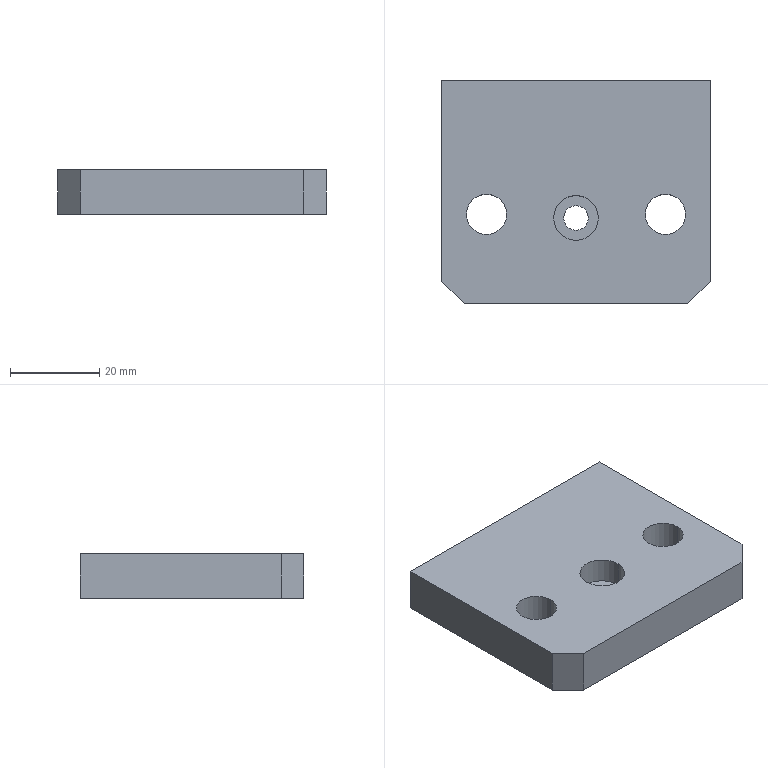Part | SolidWorks | features BaseBody 1 | 1 solid | 29 faces | box 60 x 50 x 10 mm | volume 27328 mm3 | cylinder 14 | plane 9 | cone 6 | commonest cylinder face diameters 4.2 x6 9 x4 5.5 x2 10 x2
STEP:
#1=CARTESIAN_POINT('',(-5.,-5.8,4.3));
#2=VERTEX_POINT('',#1);
#3=CARTESIAN_POINT('',(5.,-5.8,4.3));
#4=VERTEX_POINT('',#3);
#5=CARTESIAN_POINT('',(0.,-5.8,4.3));
#6=DIRECTION('',(0.,0.,1.));
#7=DIRECTION('',(1.,0.,0.));
#8=AXIS2_PLACEMENT_3D('',#5,#6,#7);
#9=CIRCLE('',#8,5.);
#10=EDGE_CURVE('',#2,#4,#9,.T.);
#11=ORIENTED_EDGE('',*,*,#10,.F.);
#12=CARTESIAN_POINT('',(-5.,-5.8,10.));
#13=VERTEX_POINT('',#12);
#14=CARTESIAN_POINT('',(-5.,-5.8,10.));
#15=DIRECTION('',(0.,0.,1.));
#16=VECTOR('',#15,1000.);
#17=LINE('',#14,#16);
#18=EDGE_CURVE('',#2,#13,#17,.T.);
#19=ORIENTED_EDGE('',*,*,#18,.T.);
#20=CARTESIAN_POINT('',(5.,-5.8,10.));
#21=VERTEX_POINT('',#20);
#22=CARTESIAN_POINT('',(0.,-5.8,10.));
#23=DIRECTION('',(0.,0.,1.));
#24=DIRECTION('',(1.,0.,0.));
#25=AXIS2_PLACEMENT_3D('',#22,#23,#24);
#26=CIRCLE('',#25,5.);
#27=EDGE_CURVE('',#13,#21,#26,.T.);
#28=ORIENTED_EDGE('',*,*,#27,.T.);
#29=CARTESIAN_POINT('',(5.,-5.8,10.));
#30=DIRECTION('',(0.,0.,1.));
#31=VECTOR('',#30,1000.);
#32=LINE('',#29,#31);
#33=EDGE_CURVE('',#4,#21,#32,.T.);
#34=ORIENTED_EDGE('',*,*,#33,.F.);
#35=EDGE_LOOP('',(#11,#19,#28,#34));
#36=FACE_OUTER_BOUND('',#35,.T.);
#37=CARTESIAN_POINT('',(0.,-5.8,10.));
#38=DIRECTION('',(0.,0.,1.));
#39=DIRECTION('',(1.,0.,0.));
#40=AXIS2_PLACEMENT_3D('',#37,#38,#39);
#41=CYLINDRICAL_SURFACE('',#40,5.);
#42=ADVANCED_FACE('',(#36),#41,.F.);
#43=CARTESIAN_POINT('',(-2.75,-5.8,0.));
#44=VERTEX_POINT('',#43);
#45=CARTESIAN_POINT('',(2.75,-5.8,0.));
#46=VERTEX_POINT('',#45);
#47=CARTESIAN_POINT('',(0.,-5.8,0.));
#48=DIRECTION('',(0.,0.,1.));
#49=DIRECTION('',(1.,0.,0.));
#50=AXIS2_PLACEMENT_3D('',#47,#48,#49);
#51=CIRCLE('',#50,2.75);
#52=EDGE_CURVE('',#44,#46,#51,.T.);
#53=ORIENTED_EDGE('',*,*,#52,.F.);
#54=CARTESIAN_POINT('',(-2.75,-5.8,4.3));
#55=VERTEX_POINT('',#54);
#56=CARTESIAN_POINT('',(-2.75,-5.8,10.));
#57=DIRECTION('',(0.,0.,1.));
#58=VECTOR('',#57,1000.);
#59=LINE('',#56,#58);
#60=EDGE_CURVE('',#44,#55,#59,.T.);
#61=ORIENTED_EDGE('',*,*,#60,.T.);
#62=CARTESIAN_POINT('',(2.75,-5.8,4.3));
#63=VERTEX_POINT('',#62);
#64=CARTESIAN_POINT('',(0.,-5.8,4.3));
#65=DIRECTION('',(0.,0.,1.));
#66=DIRECTION('',(1.,0.,0.));
#67=AXIS2_PLACEMENT_3D('',#64,#65,#66);
#68=CIRCLE('',#67,2.75);
#69=EDGE_CURVE('',#55,#63,#68,.T.);
#70=ORIENTED_EDGE('',*,*,#69,.T.);
#71=CARTESIAN_POINT('',(2.75,-5.8,10.));
#72=DIRECTION('',(0.,0.,1.));
#73=VECTOR('',#72,1000.);
#74=LINE('',#71,#73);
#75=EDGE_CURVE('',#46,#63,#74,.T.);
#76=ORIENTED_EDGE('',*,*,#75,.F.);
#77=EDGE_LOOP('',(#53,#61,#70,#76));
#78=FACE_OUTER_BOUND('',#77,.T.);
#79=CARTESIAN_POINT('',(0.,-5.8,10.));
#80=DIRECTION('',(0.,0.,1.));
#81=DIRECTION('',(1.,0.,0.));
#82=AXIS2_PLACEMENT_3D('',#79,#80,#81);
#83=CYLINDRICAL_SURFACE('',#82,2.75);
#84=ADVANCED_FACE('',(#78),#83,.F.);
#85=CARTESIAN_POINT('',(-20.,11.,2.9));
#86=VERTEX_POINT('',#85);
#87=CARTESIAN_POINT('',(-20.,11.,7.1));
#88=VERTEX_POINT('',#87);
#89=CARTESIAN_POINT('',(-20.,11.,5.));
#90=DIRECTION('',(0.,1.,0.));
#91=DIRECTION('',(0.,0.,1.));
#92=AXIS2_PLACEMENT_3D('',#89,#90,#91);
#93=CIRCLE('',#92,2.1);
#94=EDGE_CURVE('',#86,#88,#93,.T.);
#95=ORIENTED_EDGE('',*,*,#94,.F.);
#96=CARTESIAN_POINT('',(-20.,25.,2.9));
#97=VERTEX_POINT('',#96);
#98=CARTESIAN_POINT('',(-20.,25.,2.9));
#99=DIRECTION('',(0.,1.,0.));
#100=VECTOR('',#99,1000.);
#101=LINE('',#98,#100);
#102=EDGE_CURVE('',#86,#97,#101,.T.);
#103=ORIENTED_EDGE('',*,*,#102,.T.);
#104=CARTESIAN_POINT('',(-20.,25.,7.1));
#105=VERTEX_POINT('',#104);
#106=CARTESIAN_POINT('',(-20.,25.,5.));
#107=DIRECTION('',(0.,1.,0.));
#108=DIRECTION('',(0.,0.,1.));
#109=AXIS2_PLACEMENT_3D('',#106,#107,#108);
#110=CIRCLE('',#109,2.1);
#111=EDGE_CURVE('',#97,#105,#110,.T.);
#112=ORIENTED_EDGE('',*,*,#111,.T.);
#113=CARTESIAN_POINT('',(-20.,25.,7.1));
#114=DIRECTION('',(0.,1.,0.));
#115=VECTOR('',#114,1000.);
#116=LINE('',#113,#115);
#117=EDGE_CURVE('',#88,#105,#116,.T.);
#118=ORIENTED_EDGE('',*,*,#117,.F.);
#119=EDGE_LOOP('',(#95,#103,#112,#118));
#120=FACE_OUTER_BOUND('',#119,.T.);
#121=CARTESIAN_POINT('',(-20.,25.,5.));
#122=DIRECTION('',(0.,1.,0.));
#123=DIRECTION('',(0.,0.,1.));
#124=AXIS2_PLACEMENT_3D('',#121,#122,#123);
#125=CYLINDRICAL_SURFACE('',#124,2.1);
#126=ADVANCED_FACE('',(#120),#125,.F.);
#127=CARTESIAN_POINT('',(-20.,9.738,5.));
#128=VERTEX_POINT('',#127);
#129=CARTESIAN_POINT('',(-20.,11.,7.1));
#130=DIRECTION('',(0.,0.515,0.8572));
#131=VECTOR('',#130,1000.);
#132=LINE('',#129,#131);
#133=EDGE_CURVE('',#128,#88,#132,.T.);
#134=ORIENTED_EDGE('',*,*,#133,.F.);
#135=CARTESIAN_POINT('',(-20.,11.,2.9));
#136=DIRECTION('',(0.,0.515,-0.8572));
#137=VECTOR('',#136,1000.);
#138=LINE('',#135,#137);
#139=EDGE_CURVE('',#128,#86,#138,.T.);
#140=ORIENTED_EDGE('',*,*,#139,.T.);
#141=ORIENTED_EDGE('',*,*,#94,.T.);
#142=EDGE_LOOP('',(#134,#140,#141));
#143=FACE_OUTER_BOUND('',#142,.T.);
#144=CARTESIAN_POINT('',(-20.,11.,5.));
#145=DIRECTION('',(0.,1.,0.));
#146=DIRECTION('',(0.,0.,1.));
#147=AXIS2_PLACEMENT_3D('',#144,#145,#146);
#148=CONICAL_SURFACE('',#147,2.1,1.03);
#149=ADVANCED_FACE('',(#143),#148,.F.);
#150=CARTESIAN_POINT('',(0.,11.,2.9));
#151=VERTEX_POINT('',#150);
#152=CARTESIAN_POINT('',(0.,11.,7.1));
#153=VERTEX_POINT('',#152);
#154=CARTESIAN_POINT('',(0.,11.,5.));
#155=DIRECTION('',(0.,1.,0.));
#156=DIRECTION('',(0.,0.,1.));
#157=AXIS2_PLACEMENT_3D('',#154,#155,#156);
#158=CIRCLE('',#157,2.1);
#159=EDGE_CURVE('',#151,#153,#158,.T.);
#160=ORIENTED_EDGE('',*,*,#159,.F.);
#161=CARTESIAN_POINT('',(0.,25.,2.9));
#162=VERTEX_POINT('',#161);
#163=CARTESIAN_POINT('',(0.,25.,2.9));
#164=DIRECTION('',(0.,1.,0.));
#165=VECTOR('',#164,1000.);
#166=LINE('',#163,#165);
#167=EDGE_CURVE('',#151,#162,#166,.T.);
#168=ORIENTED_EDGE('',*,*,#167,.T.);
#169=CARTESIAN_POINT('',(0.,25.,7.1));
#170=VERTEX_POINT('',#169);
#171=CARTESIAN_POINT('',(0.,25.,5.));
#172=DIRECTION('',(0.,1.,0.));
#173=DIRECTION('',(0.,0.,1.));
#174=AXIS2_PLACEMENT_3D('',#171,#172,#173);
#175=CIRCLE('',#174,2.1);
#176=EDGE_CURVE('',#162,#170,#175,.T.);
#177=ORIENTED_EDGE('',*,*,#176,.T.);
#178=CARTESIAN_POINT('',(0.,25.,7.1));
#179=DIRECTION('',(0.,1.,0.));
#180=VECTOR('',#179,1000.);
#181=LINE('',#178,#180);
#182=EDGE_CURVE('',#153,#170,#181,.T.);
#183=ORIENTED_EDGE('',*,*,#182,.F.);
#184=EDGE_LOOP('',(#160,#168,#177,#183));
#185=FACE_OUTER_BOUND('',#184,.T.);
#186=CARTESIAN_POINT('',(0.,25.,5.));
#187=DIRECTION('',(0.,1.,0.));
#188=DIRECTION('',(0.,0.,1.));
#189=AXIS2_PLACEMENT_3D('',#186,#187,#188);
#190=CYLINDRICAL_SURFACE('',#189,2.1);
#191=ADVANCED_FACE('',(#185),#190,.F.);
#192=CARTESIAN_POINT('',(0.,9.738,5.));
#193=VERTEX_POINT('',#192);
#194=CARTESIAN_POINT('',(0.,11.,7.1));
#195=DIRECTION('',(0.,0.515,0.8572));
#196=VECTOR('',#195,1000.);
#197=LINE('',#194,#196);
#198=EDGE_CURVE('',#193,#153,#197,.T.);
#199=ORIENTED_EDGE('',*,*,#198,.F.);
#200=CARTESIAN_POINT('',(0.,11.,2.9));
#201=DIRECTION('',(0.,0.515,-0.8572));
#202=VECTOR('',#201,1000.);
#203=LINE('',#200,#202);
#204=EDGE_CURVE('',#193,#151,#203,.T.);
#205=ORIENTED_EDGE('',*,*,#204,.T.);
#206=ORIENTED_EDGE('',*,*,#159,.T.);
#207=EDGE_LOOP('',(#199,#205,#206));
#208=FACE_OUTER_BOUND('',#207,.T.);
#209=CARTESIAN_POINT('',(0.,11.,5.));
#210=DIRECTION('',(0.,1.,0.));
#211=DIRECTION('',(0.,0.,1.));
#212=AXIS2_PLACEMENT_3D('',#209,#210,#211);
#213=CONICAL_SURFACE('',#212,2.1,1.03);
#214=ADVANCED_FACE('',(#208),#213,.F.);
#215=CARTESIAN_POINT('',(20.,11.,2.9));
#216=VERTEX_POINT('',#215);
#217=CARTESIAN_POINT('',(20.,11.,7.1));
#218=VERTEX_POINT('',#217);
#219=CARTESIAN_POINT('',(20.,11.,5.));
#220=DIRECTION('',(0.,1.,0.));
#221=DIRECTION('',(0.,0.,1.));
#222=AXIS2_PLACEMENT_3D('',#219,#220,#221);
#223=CIRCLE('',#222,2.1);
#224=EDGE_CURVE('',#216,#218,#223,.T.);
#225=ORIENTED_EDGE('',*,*,#224,.F.);
#226=CARTESIAN_POINT('',(20.,25.,2.9));
#227=VERTEX_POINT('',#226);
#228=CARTESIAN_POINT('',(20.,25.,2.9));
#229=DIRECTION('',(0.,1.,0.));
#230=VECTOR('',#229,1000.);
#231=LINE('',#228,#230);
#232=EDGE_CURVE('',#216,#227,#231,.T.);
#233=ORIENTED_EDGE('',*,*,#232,.T.);
#234=CARTESIAN_POINT('',(20.,25.,7.1));
#235=VERTEX_POINT('',#234);
#236=CARTESIAN_POINT('',(20.,25.,5.));
#237=DIRECTION('',(0.,1.,0.));
#238=DIRECTION('',(0.,0.,1.));
#239=AXIS2_PLACEMENT_3D('',#236,#237,#238);
#240=CIRCLE('',#239,2.1);
#241=EDGE_CURVE('',#227,#235,#240,.T.);
#242=ORIENTED_EDGE('',*,*,#241,.T.);
#243=CARTESIAN_POINT('',(20.,25.,7.1));
#244=DIRECTION('',(0.,1.,0.));
#245=VECTOR('',#244,1000.);
#246=LINE('',#243,#245);
#247=EDGE_CURVE('',#218,#235,#246,.T.);
#248=ORIENTED_EDGE('',*,*,#247,.F.);
#249=EDGE_LOOP('',(#225,#233,#242,#248));
#250=FACE_OUTER_BOUND('',#249,.T.);
#251=CARTESIAN_POINT('',(20.,25.,5.));
#252=DIRECTION('',(0.,1.,0.));
#253=DIRECTION('',(0.,0.,1.));
#254=AXIS2_PLACEMENT_3D('',#251,#252,#253);
#255=CYLINDRICAL_SURFACE('',#254,2.1);
#256=ADVANCED_FACE('',(#250),#255,.F.);
#257=CARTESIAN_POINT('',(20.,9.738,5.));
#258=VERTEX_POINT('',#257);
#259=CARTESIAN_POINT('',(20.,11.,7.1));
#260=DIRECTION('',(0.,0.515,0.8572));
#261=VECTOR('',#260,1000.);
#262=LINE('',#259,#261);
#263=EDGE_CURVE('',#258,#218,#262,.T.);
#264=ORIENTED_EDGE('',*,*,#263,.F.);
#265=CARTESIAN_POINT('',(20.,11.,2.9));
#266=DIRECTION('',(0.,0.515,-0.8572));
#267=VECTOR('',#266,1000.);
#268=LINE('',#265,#267);
#269=EDGE_CURVE('',#258,#216,#268,.T.);
#270=ORIENTED_EDGE('',*,*,#269,.T.);
#271=ORIENTED_EDGE('',*,*,#224,.T.);
#272=EDGE_LOOP('',(#264,#270,#271));
#273=FACE_OUTER_BOUND('',#272,.T.);
#274=CARTESIAN_POINT('',(20.,11.,5.));
#275=DIRECTION('',(0.,1.,0.));
#276=DIRECTION('',(0.,0.,1.));
#277=AXIS2_PLACEMENT_3D('',#274,#275,#276);
#278=CONICAL_SURFACE('',#277,2.1,1.03);
#279=ADVANCED_FACE('',(#273),#278,.F.);
#280=CARTESIAN_POINT('',(-24.5,-5.,0.));
#281=VERTEX_POINT('',#280);
#282=CARTESIAN_POINT('',(-15.5,-5.,0.));
#283=VERTEX_POINT('',#282);
#284=CARTESIAN_POINT('',(-20.,-5.,0.));
#285=DIRECTION('',(0.,0.,1.));
#286=DIRECTION('',(1.,0.,0.));
#287=AXIS2_PLACEMENT_3D('',#284,#285,#286);
#288=CIRCLE('',#287,4.5);
#289=EDGE_CURVE('',#281,#283,#288,.T.);
#290=ORIENTED_EDGE('',*,*,#289,.F.);
#291=CARTESIAN_POINT('',(-24.5,-5.,10.));
#292=VERTEX_POINT('',#291);
#293=CARTESIAN_POINT('',(-24.5,-5.,10.));
#294=DIRECTION('',(0.,0.,1.));
#295=VECTOR('',#294,1000.);
#296=LINE('',#293,#295);
#297=EDGE_CURVE('',#281,#292,#296,.T.);
#298=ORIENTED_EDGE('',*,*,#297,.T.);
#299=CARTESIAN_POINT('',(-15.5,-5.,10.));
#300=VERTEX_POINT('',#299);
#301=CARTESIAN_POINT('',(-20.,-5.,10.));
#302=DIRECTION('',(0.,0.,1.));
#303=DIRECTION('',(1.,0.,0.));
#304=AXIS2_PLACEMENT_3D('',#301,#302,#303);
#305=CIRCLE('',#304,4.5);
#306=EDGE_CURVE('',#292,#300,#305,.T.);
#307=ORIENTED_EDGE('',*,*,#306,.T.);
#308=CARTESIAN_POINT('',(-15.5,-5.,10.));
#309=DIRECTION('',(0.,0.,1.));
#310=VECTOR('',#309,1000.);
#311=LINE('',#308,#310);
#312=EDGE_CURVE('',#283,#300,#311,.T.);
#313=ORIENTED_EDGE('',*,*,#312,.F.);
#314=EDGE_LOOP('',(#290,#298,#307,#313));
#315=FACE_OUTER_BOUND('',#314,.T.);
#316=CARTESIAN_POINT('',(-20.,-5.,10.));
#317=DIRECTION('',(0.,0.,1.));
#318=DIRECTION('',(1.,0.,0.));
#319=AXIS2_PLACEMENT_3D('',#316,#317,#318);
#320=CYLINDRICAL_SURFACE('',#319,4.5);
#321=ADVANCED_FACE('',(#315),#320,.F.);
#322=CARTESIAN_POINT('',(15.5,-5.,0.));
#323=VERTEX_POINT('',#322);
#324=CARTESIAN_POINT('',(24.5,-5.,0.));
#325=VERTEX_POINT('',#324);
#326=CARTESIAN_POINT('',(20.,-5.,0.));
#327=DIRECTION('',(0.,0.,1.));
#328=DIRECTION('',(1.,0.,0.));
#329=AXIS2_PLACEMENT_3D('',#326,#327,#328);
#330=CIRCLE('',#329,4.5);
#331=EDGE_CURVE('',#323,#325,#330,.T.);
#332=ORIENTED_EDGE('',*,*,#331,.F.);
#333=CARTESIAN_POINT('',(15.5,-5.,10.));
#334=VERTEX_POINT('',#333);
#335=CARTESIAN_POINT('',(15.5,-5.,10.));
#336=DIRECTION('',(0.,0.,1.));
#337=VECTOR('',#336,1000.);
#338=LINE('',#335,#337);
#339=EDGE_CURVE('',#323,#334,#338,.T.);
#340=ORIENTED_EDGE('',*,*,#339,.T.);
#341=CARTESIAN_POINT('',(24.5,-5.,10.));
#342=VERTEX_POINT('',#341);
#343=CARTESIAN_POINT('',(20.,-5.,10.));
#344=DIRECTION('',(0.,0.,1.));
#345=DIRECTION('',(1.,0.,0.));
#346=AXIS2_PLACEMENT_3D('',#343,#344,#345);
#347=CIRCLE('',#346,4.5);
#348=EDGE_CURVE('',#334,#342,#347,.T.);
#349=ORIENTED_EDGE('',*,*,#348,.T.);
#350=CARTESIAN_POINT('',(24.5,-5.,10.));
#351=DIRECTION('',(0.,0.,1.));
#352=VECTOR('',#351,1000.);
#353=LINE('',#350,#352);
#354=EDGE_CURVE('',#325,#342,#353,.T.);
#355=ORIENTED_EDGE('',*,*,#354,.F.);
#356=EDGE_LOOP('',(#332,#340,#349,#355));
#357=FACE_OUTER_BOUND('',#356,.T.);
#358=CARTESIAN_POINT('',(20.,-5.,10.));
#359=DIRECTION('',(0.,0.,1.));
#360=DIRECTION('',(1.,0.,0.));
#361=AXIS2_PLACEMENT_3D('',#358,#359,#360);
#362=CYLINDRICAL_SURFACE('',#361,4.5);
#363=ADVANCED_FACE('',(#357),#362,.F.);
#364=CARTESIAN_POINT('',(-30.,25.,0.));
#365=VERTEX_POINT('',#364);
#366=CARTESIAN_POINT('',(-30.,-20.,0.));
#367=VERTEX_POINT('',#366);
#368=CARTESIAN_POINT('',(-30.,25.,0.));
#369=DIRECTION('',(0.,-1.,0.));
#370=VECTOR('',#369,1000.);
#371=LINE('',#368,#370);
#372=EDGE_CURVE('',#365,#367,#371,.T.);
#373=ORIENTED_EDGE('',*,*,#372,.T.);
#374=CARTESIAN_POINT('',(-30.,-20.,10.));
#375=VERTEX_POINT('',#374);
#376=CARTESIAN_POINT('',(-30.,-20.,10.));
#377=DIRECTION('',(0.,0.,1.));
#378=VECTOR('',#377,1000.);
#379=LINE('',#376,#378);
#380=EDGE_CURVE('',#367,#375,#379,.T.);
#381=ORIENTED_EDGE('',*,*,#380,.T.);
#382=CARTESIAN_POINT('',(-30.,25.,10.));
#383=VERTEX_POINT('',#382);
#384=CARTESIAN_POINT('',(-30.,25.,10.));
#385=DIRECTION('',(0.,-1.,0.));
#386=VECTOR('',#385,1000.);
#387=LINE('',#384,#386);
#388=EDGE_CURVE('',#383,#375,#387,.T.);
#389=ORIENTED_EDGE('',*,*,#388,.F.);
#390=CARTESIAN_POINT('',(-30.,25.,10.));
#391=DIRECTION('',(0.,0.,-1.));
#392=VECTOR('',#391,1000.);
#393=LINE('',#390,#392);
#394=EDGE_CURVE('',#383,#365,#393,.T.);
#395=ORIENTED_EDGE('',*,*,#394,.T.);
#396=EDGE_LOOP('',(#373,#381,#389,#395));
#397=FACE_OUTER_BOUND('',#396,.T.);
#398=CARTESIAN_POINT('',(-30.,25.,10.));
#399=DIRECTION('',(1.,0.,0.));
#400=DIRECTION('',(0.,1.,0.));
#401=AXIS2_PLACEMENT_3D('',#398,#399,#400);
#402=PLANE('',#401);
#403=ADVANCED_FACE('',(#397),#402,.F.);
#404=CARTESIAN_POINT('',(-25.,-25.,10.));
#405=VERTEX_POINT('',#404);
#406=CARTESIAN_POINT('',(25.,-25.,10.));
#407=VERTEX_POINT('',#406);
#408=CARTESIAN_POINT('',(30.,-25.,10.));
#409=DIRECTION('',(1.,0.,0.));
#410=VECTOR('',#409,1000.);
#411=LINE('',#408,#410);
#412=EDGE_CURVE('',#405,#407,#411,.T.);
#413=ORIENTED_EDGE('',*,*,#412,.F.);
#414=CARTESIAN_POINT('',(-25.,-25.,0.));
#415=VERTEX_POINT('',#414);
#416=CARTESIAN_POINT('',(-25.,-25.,10.));
#417=DIRECTION('',(0.,0.,-1.));
#418=VECTOR('',#417,1000.);
#419=LINE('',#416,#418);
#420=EDGE_CURVE('',#405,#415,#419,.T.);
#421=ORIENTED_EDGE('',*,*,#420,.T.);
#422=CARTESIAN_POINT('',(25.,-25.,0.));
#423=VERTEX_POINT('',#422);
#424=CARTESIAN_POINT('',(30.,-25.,0.));
#425=DIRECTION('',(1.,0.,0.));
#426=VECTOR('',#425,1000.);
#427=LINE('',#424,#426);
#428=EDGE_CURVE('',#415,#423,#427,.T.);
#429=ORIENTED_EDGE('',*,*,#428,.T.);
#430=CARTESIAN_POINT('',(25.,-25.,10.));
#431=DIRECTION('',(0.,0.,1.));
#432=VECTOR('',#431,1000.);
#433=LINE('',#430,#432);
#434=EDGE_CURVE('',#423,#407,#433,.T.);
#435=ORIENTED_EDGE('',*,*,#434,.T.);
#436=EDGE_LOOP('',(#413,#421,#429,#435));
#437=FACE_OUTER_BOUND('',#436,.T.);
#438=CARTESIAN_POINT('',(30.,-25.,10.));
#439=DIRECTION('',(0.,1.,0.));
#440=DIRECTION('',(-1.,0.,0.));
#441=AXIS2_PLACEMENT_3D('',#438,#439,#440);
#442=PLANE('',#441);
#443=ADVANCED_FACE('',(#437),#442,.F.);
#444=CARTESIAN_POINT('',(30.,-20.,10.));
#445=VERTEX_POINT('',#444);
#446=CARTESIAN_POINT('',(30.,25.,10.));
#447=VERTEX_POINT('',#446);
#448=CARTESIAN_POINT('',(30.,25.,10.));
#449=DIRECTION('',(0.,1.,0.));
#450=VECTOR('',#449,1000.);
#451=LINE('',#448,#450);
#452=EDGE_CURVE('',#445,#447,#451,.T.);
#453=ORIENTED_EDGE('',*,*,#452,.F.);
#454=CARTESIAN_POINT('',(30.,-20.,0.));
#455=VERTEX_POINT('',#454);
#456=CARTESIAN_POINT('',(30.,-20.,10.));
#457=DIRECTION('',(0.,0.,-1.));
#458=VECTOR('',#457,1000.);
#459=LINE('',#456,#458);
#460=EDGE_CURVE('',#445,#455,#459,.T.);
#461=ORIENTED_EDGE('',*,*,#460,.T.);
#462=CARTESIAN_POINT('',(30.,25.,0.));
#463=VERTEX_POINT('',#462);
#464=CARTESIAN_POINT('',(30.,25.,0.));
#465=DIRECTION('',(0.,1.,0.));
#466=VECTOR('',#465,1000.);
#467=LINE('',#464,#466);
#468=EDGE_CURVE('',#455,#463,#467,.T.);
#469=ORIENTED_EDGE('',*,*,#468,.T.);
#470=CARTESIAN_POINT('',(30.,25.,10.));
#471=DIRECTION('',(0.,0.,-1.));
#472=VECTOR('',#471,1000.);
#473=LINE('',#470,#472);
#474=EDGE_CURVE('',#447,#463,#473,.T.);
#475=ORIENTED_EDGE('',*,*,#474,.F.);
#476=EDGE_LOOP('',(#453,#461,#469,#475));
#477=FACE_OUTER_BOUND('',#476,.T.);
#478=CARTESIAN_POINT('',(30.,25.,10.));
#479=DIRECTION('',(-1.,0.,0.));
#480=DIRECTION('',(0.,-1.,0.));
#481=AXIS2_PLACEMENT_3D('',#478,#479,#480);
#482=PLANE('',#481);
#483=ADVANCED_FACE('',(#477),#482,.F.);
#484=CARTESIAN_POINT('',(-20.,25.,5.));
#485=DIRECTION('',(0.,1.,0.));
#486=DIRECTION('',(0.,0.,1.));
#487=AXIS2_PLACEMENT_3D('',#484,#485,#486);
#488=CIRCLE('',#487,2.1);
#489=EDGE_CURVE('',#105,#97,#488,.T.);
#490=ORIENTED_EDGE('',*,*,#489,.F.);
#491=ORIENTED_EDGE('',*,*,#111,.F.);
#492=EDGE_LOOP('',(#490,#491));
#493=FACE_BOUND('',#492,.T.);
#494=CARTESIAN_POINT('',(0.,25.,5.));
#495=DIRECTION('',(0.,1.,0.));
#496=DIRECTION('',(0.,0.,1.));
#497=AXIS2_PLACEMENT_3D('',#494,#495,#496);
#498=CIRCLE('',#497,2.1);
#499=EDGE_CURVE('',#170,#162,#498,.T.);
#500=ORIENTED_EDGE('',*,*,#499,.F.);
#501=ORIENTED_EDGE('',*,*,#176,.F.);
#502=EDGE_LOOP('',(#500,#501));
#503=FACE_BOUND('',#502,.T.);
#504=CARTESIAN_POINT('',(20.,25.,5.));
#505=DIRECTION('',(0.,1.,0.));
#506=DIRECTION('',(0.,0.,1.));
#507=AXIS2_PLACEMENT_3D('',#504,#505,#506);
#508=CIRCLE('',#507,2.1);
#509=EDGE_CURVE('',#235,#227,#508,.T.);
#510=ORIENTED_EDGE('',*,*,#509,.F.);
#511=ORIENTED_EDGE('',*,*,#241,.F.);
#512=EDGE_LOOP('',(#510,#511));
#513=FACE_BOUND('',#512,.T.);
#514=CARTESIAN_POINT('',(30.,25.,0.));
#515=DIRECTION('',(-1.,0.,0.));
#516=VECTOR('',#515,1000.);
#517=LINE('',#514,#516);
#518=EDGE_CURVE('',#463,#365,#517,.T.);
#519=ORIENTED_EDGE('',*,*,#518,.T.);
#520=ORIENTED_EDGE('',*,*,#394,.F.);
#521=CARTESIAN_POINT('',(30.,25.,10.));
#522=DIRECTION('',(-1.,0.,0.));
#523=VECTOR('',#522,1000.);
#524=LINE('',#521,#523);
#525=EDGE_CURVE('',#447,#383,#524,.T.);
#526=ORIENTED_EDGE('',*,*,#525,.F.);
#527=ORIENTED_EDGE('',*,*,#474,.T.);
#528=EDGE_LOOP('',(#519,#520,#526,#527));
#529=FACE_OUTER_BOUND('',#528,.T.);
#530=CARTESIAN_POINT('',(30.,25.,10.));
#531=DIRECTION('',(0.,-1.,0.));
#532=DIRECTION('',(1.,0.,0.));
#533=AXIS2_PLACEMENT_3D('',#530,#531,#532);
#534=PLANE('',#533);
#535=ADVANCED_FACE('',(#493,#503,#513,#529),#534,.F.);
#536=CARTESIAN_POINT('',(0.,-5.8,10.));
#537=DIRECTION('',(0.,0.,1.));
#538=DIRECTION('',(1.,0.,0.));
#539=AXIS2_PLACEMENT_3D('',#536,#537,#538);
#540=CIRCLE('',#539,5.);
#541=EDGE_CURVE('',#21,#13,#540,.T.);
#542=ORIENTED_EDGE('',*,*,#541,.F.);
#543=ORIENTED_EDGE('',*,*,#27,.F.);
#544=EDGE_LOOP('',(#542,#543));
#545=FACE_BOUND('',#544,.T.);
#546=CARTESIAN_POINT('',(-20.,-5.,10.));
#547=DIRECTION('',(0.,0.,1.));
#548=DIRECTION('',(1.,0.,0.));
#549=AXIS2_PLACEMENT_3D('',#546,#547,#548);
#550=CIRCLE('',#549,4.5);
#551=EDGE_CURVE('',#300,#292,#550,.T.);
#552=ORIENTED_EDGE('',*,*,#551,.F.);
#553=ORIENTED_EDGE('',*,*,#306,.F.);
#554=EDGE_LOOP('',(#552,#553));
#555=FACE_BOUND('',#554,.T.);
#556=CARTESIAN_POINT('',(20.,-5.,10.));
#557=DIRECTION('',(0.,0.,1.));
#558=DIRECTION('',(1.,0.,0.));
#559=AXIS2_PLACEMENT_3D('',#556,#557,#558);
#560=CIRCLE('',#559,4.5);
#561=EDGE_CURVE('',#342,#334,#560,.T.);
#562=ORIENTED_EDGE('',*,*,#561,.F.);
#563=ORIENTED_EDGE('',*,*,#348,.F.);
#564=EDGE_LOOP('',(#562,#563));
#565=FACE_BOUND('',#564,.T.);
#566=ORIENTED_EDGE('',*,*,#388,.T.);
#567=CARTESIAN_POINT('',(-25.,-25.,10.));
#568=DIRECTION('',(0.7071,-0.7071,0.));
#569=VECTOR('',#568,1000.);
#570=LINE('',#567,#569);
#571=EDGE_CURVE('',#375,#405,#570,.T.);
#572=ORIENTED_EDGE('',*,*,#571,.T.);
#573=ORIENTED_EDGE('',*,*,#412,.T.);
#574=CARTESIAN_POINT('',(30.,-20.,10.));
#575=DIRECTION('',(0.7071,0.7071,0.));
#576=VECTOR('',#575,1000.);
#577=LINE('',#574,#576);
#578=EDGE_CURVE('',#407,#445,#577,.T.);
#579=ORIENTED_EDGE('',*,*,#578,.T.);
#580=ORIENTED_EDGE('',*,*,#452,.T.);
#581=ORIENTED_EDGE('',*,*,#525,.T.);
#582=EDGE_LOOP('',(#566,#572,#573,#579,#580,#581));
#583=FACE_OUTER_BOUND('',#582,.T.);
#584=CARTESIAN_POINT('',(0.,0.,10.));
#585=DIRECTION('',(0.,0.,-1.));
#586=DIRECTION('',(-1.,0.,0.));
#587=AXIS2_PLACEMENT_3D('',#584,#585,#586);
#588=PLANE('',#587);
#589=ADVANCED_FACE('',(#545,#555,#565,#583),#588,.F.);
#590=CARTESIAN_POINT('',(0.,-5.8,0.));
#591=DIRECTION('',(0.,0.,1.));
#592=DIRECTION('',(1.,0.,0.));
#593=AXIS2_PLACEMENT_3D('',#590,#591,#592);
#594=CIRCLE('',#593,2.75);
#595=EDGE_CURVE('',#46,#44,#594,.T.);
#596=ORIENTED_EDGE('',*,*,#595,.T.);
#597=ORIENTED_EDGE('',*,*,#52,.T.);
#598=EDGE_LOOP('',(#596,#597));
#599=FACE_BOUND('',#598,.T.);
#600=CARTESIAN_POINT('',(-20.,-5.,0.));
#601=DIRECTION('',(0.,0.,1.));
#602=DIRECTION('',(1.,0.,0.));
#603=AXIS2_PLACEMENT_3D('',#600,#601,#602);
#604=CIRCLE('',#603,4.5);
#605=EDGE_CURVE('',#283,#281,#604,.T.);
#606=ORIENTED_EDGE('',*,*,#605,.T.);
#607=ORIENTED_EDGE('',*,*,#289,.T.);
#608=EDGE_LOOP('',(#606,#607));
#609=FACE_BOUND('',#608,.T.);
#610=CARTESIAN_POINT('',(20.,-5.,0.));
#611=DIRECTION('',(0.,0.,1.));
#612=DIRECTION('',(1.,0.,0.));
#613=AXIS2_PLACEMENT_3D('',#610,#611,#612);
#614=CIRCLE('',#613,4.5);
#615=EDGE_CURVE('',#325,#323,#614,.T.);
#616=ORIENTED_EDGE('',*,*,#615,.T.);
#617=ORIENTED_EDGE('',*,*,#331,.T.);
#618=EDGE_LOOP('',(#616,#617));
#619=FACE_BOUND('',#618,.T.);
#620=ORIENTED_EDGE('',*,*,#428,.F.);
#621=CARTESIAN_POINT('',(-25.,-25.,0.));
#622=DIRECTION('',(-0.7071,0.7071,0.));
#623=VECTOR('',#622,1000.);
#624=LINE('',#621,#623);
#625=EDGE_CURVE('',#415,#367,#624,.T.);
#626=ORIENTED_EDGE('',*,*,#625,.T.);
#627=ORIENTED_EDGE('',*,*,#372,.F.);
#628=ORIENTED_EDGE('',*,*,#518,.F.);
#629=ORIENTED_EDGE('',*,*,#468,.F.);
#630=CARTESIAN_POINT('',(25.,-25.,0.));
#631=DIRECTION('',(-0.7071,-0.7071,0.));
#632=VECTOR('',#631,1000.);
#633=LINE('',#630,#632);
#634=EDGE_CURVE('',#455,#423,#633,.T.);
#635=ORIENTED_EDGE('',*,*,#634,.T.);
#636=EDGE_LOOP('',(#620,#626,#627,#628,#629,#635));
#637=FACE_OUTER_BOUND('',#636,.T.);
#638=CARTESIAN_POINT('',(0.,0.,0.));
#639=DIRECTION('',(0.,0.,-1.));
#640=DIRECTION('',(-1.,0.,0.));
#641=AXIS2_PLACEMENT_3D('',#638,#639,#640);
#642=PLANE('',#641);
#643=ADVANCED_FACE('',(#599,#609,#619,#637),#642,.T.);
#644=ORIENTED_EDGE('',*,*,#571,.F.);
#645=ORIENTED_EDGE('',*,*,#380,.F.);
#646=ORIENTED_EDGE('',*,*,#625,.F.);
#647=ORIENTED_EDGE('',*,*,#420,.F.);
#648=EDGE_LOOP('',(#644,#645,#646,#647));
#649=FACE_OUTER_BOUND('',#648,.T.);
#650=CARTESIAN_POINT('',(-25.,-25.,10.));
#651=DIRECTION('',(0.7071,0.7071,0.));
#652=DIRECTION('',(0.,0.,-1.));
#653=AXIS2_PLACEMENT_3D('',#650,#651,#652);
#654=PLANE('',#653);
#655=ADVANCED_FACE('',(#649),#654,.F.);
#656=ORIENTED_EDGE('',*,*,#578,.F.);
#657=ORIENTED_EDGE('',*,*,#434,.F.);
#658=ORIENTED_EDGE('',*,*,#634,.F.);
#659=ORIENTED_EDGE('',*,*,#460,.F.);
#660=EDGE_LOOP('',(#656,#657,#658,#659));
#661=FACE_OUTER_BOUND('',#660,.T.);
#662=CARTESIAN_POINT('',(30.,-20.,10.));
#663=DIRECTION('',(-0.7071,0.7071,0.));
#664=DIRECTION('',(0.,0.,-1.));
#665=AXIS2_PLACEMENT_3D('',#662,#663,#664);
#666=PLANE('',#665);
#667=ADVANCED_FACE('',(#661),#666,.F.);
#668=ORIENTED_EDGE('',*,*,#339,.F.);
#669=ORIENTED_EDGE('',*,*,#615,.F.);
#670=ORIENTED_EDGE('',*,*,#354,.T.);
#671=ORIENTED_EDGE('',*,*,#561,.T.);
#672=EDGE_LOOP('',(#668,#669,#670,#671));
#673=FACE_OUTER_BOUND('',#672,.T.);
#674=CARTESIAN_POINT('',(20.,-5.,10.));
#675=DIRECTION('',(0.,0.,1.));
#676=DIRECTION('',(1.,0.,0.));
#677=AXIS2_PLACEMENT_3D('',#674,#675,#676);
#678=CYLINDRICAL_SURFACE('',#677,4.5);
#679=ADVANCED_FACE('',(#673),#678,.F.);
#680=ORIENTED_EDGE('',*,*,#297,.F.);
#681=ORIENTED_EDGE('',*,*,#605,.F.);
#682=ORIENTED_EDGE('',*,*,#312,.T.);
#683=ORIENTED_EDGE('',*,*,#551,.T.);
#684=EDGE_LOOP('',(#680,#681,#682,#683));
#685=FACE_OUTER_BOUND('',#684,.T.);
#686=CARTESIAN_POINT('',(-20.,-5.,10.));
#687=DIRECTION('',(0.,0.,1.));
#688=DIRECTION('',(1.,0.,0.));
#689=AXIS2_PLACEMENT_3D('',#686,#687,#688);
#690=CYLINDRICAL_SURFACE('',#689,4.5);
#691=ADVANCED_FACE('',(#685),#690,.F.);
#692=ORIENTED_EDGE('',*,*,#269,.F.);
#693=ORIENTED_EDGE('',*,*,#263,.T.);
#694=CARTESIAN_POINT('',(20.,11.,5.));
#695=DIRECTION('',(0.,1.,0.));
#696=DIRECTION('',(0.,0.,1.));
#697=AXIS2_PLACEMENT_3D('',#694,#695,#696);
#698=CIRCLE('',#697,2.1);
#699=EDGE_CURVE('',#218,#216,#698,.T.);
#700=ORIENTED_EDGE('',*,*,#699,.T.);
#701=EDGE_LOOP('',(#692,#693,#700));
#702=FACE_OUTER_BOUND('',#701,.T.);
#703=CARTESIAN_POINT('',(20.,11.,5.));
#704=DIRECTION('',(0.,1.,0.));
#705=DIRECTION('',(0.,0.,1.));
#706=AXIS2_PLACEMENT_3D('',#703,#704,#705);
#707=CONICAL_SURFACE('',#706,2.1,1.03);
#708=ADVANCED_FACE('',(#702),#707,.F.);
#709=ORIENTED_EDGE('',*,*,#232,.F.);
#710=ORIENTED_EDGE('',*,*,#699,.F.);
#711=ORIENTED_EDGE('',*,*,#247,.T.);
#712=ORIENTED_EDGE('',*,*,#509,.T.);
#713=EDGE_LOOP('',(#709,#710,#711,#712));
#714=FACE_OUTER_BOUND('',#713,.T.);
#715=CARTESIAN_POINT('',(20.,25.,5.));
#716=DIRECTION('',(0.,1.,0.));
#717=DIRECTION('',(0.,0.,1.));
#718=AXIS2_PLACEMENT_3D('',#715,#716,#717);
#719=CYLINDRICAL_SURFACE('',#718,2.1);
#720=ADVANCED_FACE('',(#714),#719,.F.);
#721=ORIENTED_EDGE('',*,*,#204,.F.);
#722=ORIENTED_EDGE('',*,*,#198,.T.);
#723=CARTESIAN_POINT('',(0.,11.,5.));
#724=DIRECTION('',(0.,1.,0.));
#725=DIRECTION('',(0.,0.,1.));
#726=AXIS2_PLACEMENT_3D('',#723,#724,#725);
#727=CIRCLE('',#726,2.1);
#728=EDGE_CURVE('',#153,#151,#727,.T.);
#729=ORIENTED_EDGE('',*,*,#728,.T.);
#730=EDGE_LOOP('',(#721,#722,#729));
#731=FACE_OUTER_BOUND('',#730,.T.);
#732=CARTESIAN_POINT('',(0.,11.,5.));
#733=DIRECTION('',(0.,1.,0.));
#734=DIRECTION('',(0.,0.,1.));
#735=AXIS2_PLACEMENT_3D('',#732,#733,#734);
#736=CONICAL_SURFACE('',#735,2.1,1.03);
#737=ADVANCED_FACE('',(#731),#736,.F.);
#738=ORIENTED_EDGE('',*,*,#167,.F.);
#739=ORIENTED_EDGE('',*,*,#728,.F.);
#740=ORIENTED_EDGE('',*,*,#182,.T.);
#741=ORIENTED_EDGE('',*,*,#499,.T.);
#742=EDGE_LOOP('',(#738,#739,#740,#741));
#743=FACE_OUTER_BOUND('',#742,.T.);
#744=CARTESIAN_POINT('',(0.,25.,5.));
#745=DIRECTION('',(0.,1.,0.));
#746=DIRECTION('',(0.,0.,1.));
#747=AXIS2_PLACEMENT_3D('',#744,#745,#746);
#748=CYLINDRICAL_SURFACE('',#747,2.1);
#749=ADVANCED_FACE('',(#743),#748,.F.);
#750=ORIENTED_EDGE('',*,*,#139,.F.);
#751=ORIENTED_EDGE('',*,*,#133,.T.);
#752=CARTESIAN_POINT('',(-20.,11.,5.));
#753=DIRECTION('',(0.,1.,0.));
#754=DIRECTION('',(0.,0.,1.));
#755=AXIS2_PLACEMENT_3D('',#752,#753,#754);
#756=CIRCLE('',#755,2.1);
#757=EDGE_CURVE('',#88,#86,#756,.T.);
#758=ORIENTED_EDGE('',*,*,#757,.T.);
#759=EDGE_LOOP('',(#750,#751,#758));
#760=FACE_OUTER_BOUND('',#759,.T.);
#761=CARTESIAN_POINT('',(-20.,11.,5.));
#762=DIRECTION('',(0.,1.,0.));
#763=DIRECTION('',(0.,0.,1.));
#764=AXIS2_PLACEMENT_3D('',#761,#762,#763);
#765=CONICAL_SURFACE('',#764,2.1,1.03);
#766=ADVANCED_FACE('',(#760),#765,.F.);
#767=ORIENTED_EDGE('',*,*,#102,.F.);
#768=ORIENTED_EDGE('',*,*,#757,.F.);
#769=ORIENTED_EDGE('',*,*,#117,.T.);
#770=ORIENTED_EDGE('',*,*,#489,.T.);
#771=EDGE_LOOP('',(#767,#768,#769,#770));
#772=FACE_OUTER_BOUND('',#771,.T.);
#773=CARTESIAN_POINT('',(-20.,25.,5.));
#774=DIRECTION('',(0.,1.,0.));
#775=DIRECTION('',(0.,0.,1.));
#776=AXIS2_PLACEMENT_3D('',#773,#774,#775);
#777=CYLINDRICAL_SURFACE('',#776,2.1);
#778=ADVANCED_FACE('',(#772),#777,.F.);
#779=ORIENTED_EDGE('',*,*,#60,.F.);
#780=ORIENTED_EDGE('',*,*,#595,.F.);
#781=ORIENTED_EDGE('',*,*,#75,.T.);
#782=CARTESIAN_POINT('',(0.,-5.8,4.3));
#783=DIRECTION('',(0.,0.,1.));
#784=DIRECTION('',(1.,0.,0.));
#785=AXIS2_PLACEMENT_3D('',#782,#783,#784);
#786=CIRCLE('',#785,2.75);
#787=EDGE_CURVE('',#63,#55,#786,.T.);
#788=ORIENTED_EDGE('',*,*,#787,.T.);
#789=EDGE_LOOP('',(#779,#780,#781,#788));
#790=FACE_OUTER_BOUND('',#789,.T.);
#791=CARTESIAN_POINT('',(0.,-5.8,10.));
#792=DIRECTION('',(0.,0.,1.));
#793=DIRECTION('',(1.,0.,0.));
#794=AXIS2_PLACEMENT_3D('',#791,#792,#793);
#795=CYLINDRICAL_SURFACE('',#794,2.75);
#796=ADVANCED_FACE('',(#790),#795,.F.);
#797=ORIENTED_EDGE('',*,*,#787,.F.);
#798=ORIENTED_EDGE('',*,*,#69,.F.);
#799=EDGE_LOOP('',(#797,#798));
#800=FACE_BOUND('',#799,.T.);
#801=CARTESIAN_POINT('',(0.,-5.8,4.3));
#802=DIRECTION('',(0.,0.,1.));
#803=DIRECTION('',(1.,0.,0.));
#804=AXIS2_PLACEMENT_3D('',#801,#802,#803);
#805=CIRCLE('',#804,5.);
#806=EDGE_CURVE('',#4,#2,#805,.T.);
#807=ORIENTED_EDGE('',*,*,#806,.T.);
#808=ORIENTED_EDGE('',*,*,#10,.T.);
#809=EDGE_LOOP('',(#807,#808));
#810=FACE_OUTER_BOUND('',#809,.T.);
#811=CARTESIAN_POINT('',(2.75,-5.8,4.3));
#812=DIRECTION('',(0.,0.,-1.));
#813=DIRECTION('',(-1.,0.,0.));
#814=AXIS2_PLACEMENT_3D('',#811,#812,#813);
#815=PLANE('',#814);
#816=ADVANCED_FACE('',(#800,#810),#815,.F.);
#817=ORIENTED_EDGE('',*,*,#18,.F.);
#818=ORIENTED_EDGE('',*,*,#806,.F.);
#819=ORIENTED_EDGE('',*,*,#33,.T.);
#820=ORIENTED_EDGE('',*,*,#541,.T.);
#821=EDGE_LOOP('',(#817,#818,#819,#820));
#822=FACE_OUTER_BOUND('',#821,.T.);
#823=CARTESIAN_POINT('',(0.,-5.8,10.));
#824=DIRECTION('',(0.,0.,1.));
#825=DIRECTION('',(1.,0.,0.));
#826=AXIS2_PLACEMENT_3D('',#823,#824,#825);
#827=CYLINDRICAL_SURFACE('',#826,5.);
#828=ADVANCED_FACE('',(#822),#827,.F.);
#829=CLOSED_SHELL('',(#42,#84,#126,#149,#191,#214,#256,#279,#321,#363,#403,#443,#483,#535,#589,#643,#655,#667,#679,#691,#708,#720,#737,#749,#766,#778,#796,#816,#828));
#830=MANIFOLD_SOLID_BREP('',#829);
#831=CARTESIAN_POINT('',(0.,0.,0.));
#832=DIRECTION('',(0.,0.,1.));
#833=DIRECTION('',(1.,0.,0.));
#834=AXIS2_PLACEMENT_3D('',#831,#832,#833);
#835=(LENGTH_UNIT()NAMED_UNIT(*)SI_UNIT(.MILLI.,.METRE.));
#836=UNCERTAINTY_MEASURE_WITH_UNIT(LENGTH_MEASURE(0.00001),#835,'','');
#837=(NAMED_UNIT(*)PLANE_ANGLE_UNIT()SI_UNIT($,.RADIAN.));
#838=(NAMED_UNIT(*)SI_UNIT($,.STERADIAN.)SOLID_ANGLE_UNIT());
#839=(GEOMETRIC_REPRESENTATION_CONTEXT(3)GLOBAL_UNCERTAINTY_ASSIGNED_CONTEXT((#836))GLOBAL_UNIT_ASSIGNED_CONTEXT((#835,#837,#838))REPRESENTATION_CONTEXT('',''));
#840=ADVANCED_BREP_SHAPE_REPRESENTATION('',(#830,#834),#839);